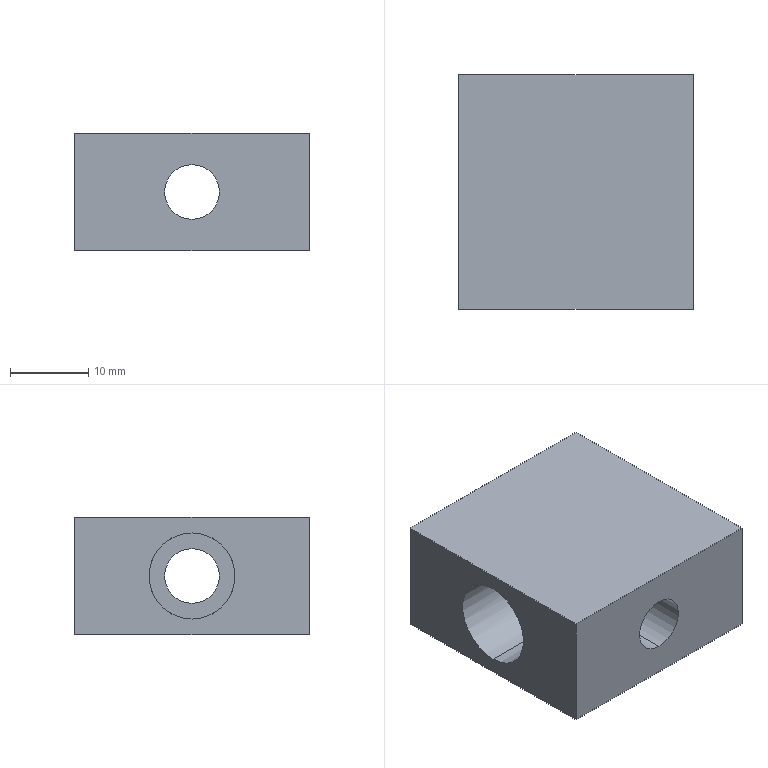Part | SolidWorks | features BaseBody 1 | 1 solid | 24 faces | box 30 x 30 x 15 mm | volume 9216 mm3 | cylinder 16 | plane 8 | commonest cylinder face diameters 11 x8 3.3 x4 7 x4
STEP:
#1=CARTESIAN_POINT('',(9.65,15.,2.));
#2=VERTEX_POINT('',#1);
#3=CARTESIAN_POINT('',(6.35,15.,2.));
#4=VERTEX_POINT('',#3);
#5=CARTESIAN_POINT('',(9.65,15.,2.));
#6=CARTESIAN_POINT('',(9.65,14.89,2.));
#7=CARTESIAN_POINT('',(9.639,14.783,2.003));
#8=CARTESIAN_POINT('',(9.597,14.571,2.016));
#9=CARTESIAN_POINT('',(9.565,14.466,2.025));
#10=CARTESIAN_POINT('',(9.482,14.266,2.048));
#11=CARTESIAN_POINT('',(9.431,14.172,2.062));
#12=CARTESIAN_POINT('',(9.311,13.993,2.092));
#13=CARTESIAN_POINT('',(9.242,13.909,2.109));
#14=CARTESIAN_POINT('',(9.015,13.682,2.158));
#15=CARTESIAN_POINT('',(8.832,13.559,2.191));
#16=CARTESIAN_POINT('',(8.436,13.394,2.239));
#17=CARTESIAN_POINT('',(8.218,13.35,2.253));
#18=CARTESIAN_POINT('',(7.893,13.35,2.253));
#19=CARTESIAN_POINT('',(7.783,13.361,2.25));
#20=CARTESIAN_POINT('',(7.571,13.403,2.237));
#21=CARTESIAN_POINT('',(7.468,13.434,2.227));
#22=CARTESIAN_POINT('',(7.167,13.559,2.191));
#23=CARTESIAN_POINT('',(6.986,13.681,2.158));
#24=CARTESIAN_POINT('',(6.758,13.909,2.109));
#25=CARTESIAN_POINT('',(6.69,13.991,2.093));
#26=CARTESIAN_POINT('',(6.57,14.169,2.062));
#27=CARTESIAN_POINT('',(6.518,14.266,2.048));
#28=CARTESIAN_POINT('',(6.394,14.564,2.014));
#29=CARTESIAN_POINT('',(6.35,14.781,2.));
#30=CARTESIAN_POINT('',(6.35,15.,2.));
#31=B_SPLINE_CURVE_WITH_KNOTS('',3,(#5,#6,#7,#8,#9,#10,#11,#12,#13,#14,#15,#16,#17,#18,#19,#20,#21,#22,#23,#24,#25,#26,#27,#28,#29,#30),.UNSPECIFIED.,.F.,.F.,(4,2,2,2,2,2,2,2,2,2,2,2,4),(0.,0.0003242,0.0006484,0.0009725,0.001297,0.001945,0.002593,0.002918,0.003242,0.00389,0.004214,0.004539,0.005187),.UNSPECIFIED.);
#32=EDGE_CURVE('',#2,#4,#31,.T.);
#33=ORIENTED_EDGE('',*,*,#32,.F.);
#34=CARTESIAN_POINT('',(9.65,15.,0.));
#35=VERTEX_POINT('',#34);
#36=CARTESIAN_POINT('',(9.65,15.,0.));
#37=DIRECTION('',(0.,0.,-1.));
#38=VECTOR('',#37,1000.);
#39=LINE('',#36,#38);
#40=EDGE_CURVE('',#2,#35,#39,.T.);
#41=ORIENTED_EDGE('',*,*,#40,.T.);
#42=CARTESIAN_POINT('',(6.35,15.,0.));
#43=VERTEX_POINT('',#42);
#44=CARTESIAN_POINT('',(8.,15.,0.));
#45=DIRECTION('',(0.,0.,-1.));
#46=DIRECTION('',(-1.,0.,0.));
#47=AXIS2_PLACEMENT_3D('',#44,#45,#46);
#48=CIRCLE('',#47,1.65);
#49=EDGE_CURVE('',#35,#43,#48,.T.);
#50=ORIENTED_EDGE('',*,*,#49,.T.);
#51=CARTESIAN_POINT('',(6.35,15.,0.));
#52=DIRECTION('',(0.,0.,-1.));
#53=VECTOR('',#52,1000.);
#54=LINE('',#51,#53);
#55=EDGE_CURVE('',#4,#43,#54,.T.);
#56=ORIENTED_EDGE('',*,*,#55,.F.);
#57=EDGE_LOOP('',(#33,#41,#50,#56));
#58=FACE_OUTER_BOUND('',#57,.T.);
#59=CARTESIAN_POINT('',(8.,15.,0.));
#60=DIRECTION('',(0.,0.,-1.));
#61=DIRECTION('',(-1.,0.,0.));
#62=AXIS2_PLACEMENT_3D('',#59,#60,#61);
#63=CYLINDRICAL_SURFACE('',#62,1.65);
#64=ADVANCED_FACE('',(#58),#63,.F.);
#65=CARTESIAN_POINT('',(16.65,22.,2.253));
#66=VERTEX_POINT('',#65);
#67=CARTESIAN_POINT('',(15.,20.35,2.));
#68=VERTEX_POINT('',#67);
#69=CARTESIAN_POINT('',(16.65,22.,2.253));
#70=CARTESIAN_POINT('',(16.65,21.89,2.253));
#71=CARTESIAN_POINT('',(16.639,21.783,2.25));
#72=CARTESIAN_POINT('',(16.597,21.571,2.237));
#73=CARTESIAN_POINT('',(16.565,21.466,2.227));
#74=CARTESIAN_POINT('',(16.482,21.267,2.203));
#75=CARTESIAN_POINT('',(16.431,21.172,2.189));
#76=CARTESIAN_POINT('',(16.312,20.993,2.158));
#77=CARTESIAN_POINT('',(16.243,20.909,2.142));
#78=CARTESIAN_POINT('',(16.016,20.682,2.092));
#79=CARTESIAN_POINT('',(15.833,20.56,2.06));
#80=CARTESIAN_POINT('',(15.437,20.394,2.014));
#81=CARTESIAN_POINT('',(15.219,20.35,2.));
#82=CARTESIAN_POINT('',(15.,20.35,2.));
#83=B_SPLINE_CURVE_WITH_KNOTS('',3,(#69,#70,#71,#72,#73,#74,#75,#76,#77,#78,#79,#80,#81,#82),.UNSPECIFIED.,.F.,.F.,(4,2,2,2,2,2,4),(0.,0.0003241,0.0006481,0.0009722,0.001296,0.001944,0.002593),.UNSPECIFIED.);
#84=EDGE_CURVE('',#66,#68,#83,.T.);
#85=ORIENTED_EDGE('',*,*,#84,.F.);
#86=CARTESIAN_POINT('',(16.65,22.,0.));
#87=VERTEX_POINT('',#86);
#88=CARTESIAN_POINT('',(16.65,22.,0.));
#89=DIRECTION('',(0.,0.,-1.));
#90=VECTOR('',#89,1000.);
#91=LINE('',#88,#90);
#92=EDGE_CURVE('',#66,#87,#91,.T.);
#93=ORIENTED_EDGE('',*,*,#92,.T.);
#94=CARTESIAN_POINT('',(13.35,22.,0.));
#95=VERTEX_POINT('',#94);
#96=CARTESIAN_POINT('',(15.,22.,0.));
#97=DIRECTION('',(0.,0.,-1.));
#98=DIRECTION('',(-1.,0.,0.));
#99=AXIS2_PLACEMENT_3D('',#96,#97,#98);
#100=CIRCLE('',#99,1.65);
#101=EDGE_CURVE('',#87,#95,#100,.T.);
#102=ORIENTED_EDGE('',*,*,#101,.T.);
#103=CARTESIAN_POINT('',(13.35,22.,2.253));
#104=VERTEX_POINT('',#103);
#105=CARTESIAN_POINT('',(13.35,22.,0.));
#106=DIRECTION('',(0.,0.,-1.));
#107=VECTOR('',#106,1000.);
#108=LINE('',#105,#107);
#109=EDGE_CURVE('',#104,#95,#108,.T.);
#110=ORIENTED_EDGE('',*,*,#109,.F.);
#111=CARTESIAN_POINT('',(15.,20.35,2.));
#112=CARTESIAN_POINT('',(14.89,20.35,2.));
#113=CARTESIAN_POINT('',(14.783,20.361,2.003));
#114=CARTESIAN_POINT('',(14.571,20.403,2.016));
#115=CARTESIAN_POINT('',(14.466,20.435,2.025));
#116=CARTESIAN_POINT('',(14.267,20.518,2.048));
#117=CARTESIAN_POINT('',(14.172,20.569,2.062));
#118=CARTESIAN_POINT('',(13.993,20.688,2.092));
#119=CARTESIAN_POINT('',(13.909,20.758,2.109));
#120=CARTESIAN_POINT('',(13.682,20.984,2.158));
#121=CARTESIAN_POINT('',(13.56,21.167,2.191));
#122=CARTESIAN_POINT('',(13.394,21.563,2.239));
#123=CARTESIAN_POINT('',(13.35,21.781,2.253));
#124=CARTESIAN_POINT('',(13.35,22.,2.253));
#125=B_SPLINE_CURVE_WITH_KNOTS('',3,(#111,#112,#113,#114,#115,#116,#117,#118,#119,#120,#121,#122,#123,#124),.UNSPECIFIED.,.F.,.F.,(4,2,2,2,2,2,4),(0.002593,0.002917,0.003241,0.003565,0.003889,0.004537,0.005185),.UNSPECIFIED.);
#126=EDGE_CURVE('',#68,#104,#125,.T.);
#127=ORIENTED_EDGE('',*,*,#126,.F.);
#128=EDGE_LOOP('',(#85,#93,#102,#110,#127));
#129=FACE_OUTER_BOUND('',#128,.T.);
#130=CARTESIAN_POINT('',(15.,22.,0.));
#131=DIRECTION('',(0.,0.,-1.));
#132=DIRECTION('',(-1.,0.,0.));
#133=AXIS2_PLACEMENT_3D('',#130,#131,#132);
#134=CYLINDRICAL_SURFACE('',#133,1.65);
#135=ADVANCED_FACE('',(#129),#134,.F.);
#136=CARTESIAN_POINT('',(30.,15.,4.));
#137=VERTEX_POINT('',#136);
#138=CARTESIAN_POINT('',(30.,15.,11.));
#139=VERTEX_POINT('',#138);
#140=CARTESIAN_POINT('',(30.,15.,7.5));
#141=DIRECTION('',(-1.,0.,0.));
#142=DIRECTION('',(0.,0.,1.));
#143=AXIS2_PLACEMENT_3D('',#140,#141,#142);
#144=CIRCLE('',#143,3.5);
#145=EDGE_CURVE('',#137,#139,#144,.T.);
#146=ORIENTED_EDGE('',*,*,#145,.F.);
#147=CARTESIAN_POINT('',(25.,15.,4.));
#148=VERTEX_POINT('',#147);
#149=CARTESIAN_POINT('',(0.,15.,4.));
#150=DIRECTION('',(-1.,0.,0.));
#151=VECTOR('',#150,1000.);
#152=LINE('',#149,#151);
#153=EDGE_CURVE('',#137,#148,#152,.T.);
#154=ORIENTED_EDGE('',*,*,#153,.T.);
#155=CARTESIAN_POINT('',(25.,15.,11.));
#156=VERTEX_POINT('',#155);
#157=CARTESIAN_POINT('',(25.,15.,7.5));
#158=DIRECTION('',(-1.,0.,0.));
#159=DIRECTION('',(0.,0.,1.));
#160=AXIS2_PLACEMENT_3D('',#157,#158,#159);
#161=CIRCLE('',#160,3.5);
#162=EDGE_CURVE('',#148,#156,#161,.T.);
#163=ORIENTED_EDGE('',*,*,#162,.T.);
#164=CARTESIAN_POINT('',(0.,15.,11.));
#165=DIRECTION('',(-1.,0.,0.));
#166=VECTOR('',#165,1000.);
#167=LINE('',#164,#166);
#168=EDGE_CURVE('',#139,#156,#167,.T.);
#169=ORIENTED_EDGE('',*,*,#168,.F.);
#170=EDGE_LOOP('',(#146,#154,#163,#169));
#171=FACE_OUTER_BOUND('',#170,.T.);
#172=CARTESIAN_POINT('',(0.,15.,7.5));
#173=DIRECTION('',(-1.,0.,0.));
#174=DIRECTION('',(0.,0.,1.));
#175=AXIS2_PLACEMENT_3D('',#172,#173,#174);
#176=CYLINDRICAL_SURFACE('',#175,3.5);
#177=ADVANCED_FACE('',(#171),#176,.F.);
#178=CARTESIAN_POINT('',(25.,15.,2.));
#179=VERTEX_POINT('',#178);
#180=CARTESIAN_POINT('',(25.,15.,13.));
#181=VERTEX_POINT('',#180);
#182=CARTESIAN_POINT('',(25.,15.,7.5));
#183=DIRECTION('',(-1.,0.,0.));
#184=DIRECTION('',(0.,0.,1.));
#185=AXIS2_PLACEMENT_3D('',#182,#183,#184);
#186=CIRCLE('',#185,5.5);
#187=EDGE_CURVE('',#179,#181,#186,.T.);
#188=ORIENTED_EDGE('',*,*,#187,.F.);
#189=CARTESIAN_POINT('',(15.,15.,2.));
#190=VERTEX_POINT('',#189);
#191=CARTESIAN_POINT('',(0.,15.,2.));
#192=DIRECTION('',(-1.,0.,0.));
#193=VECTOR('',#192,1000.);
#194=LINE('',#191,#193);
#195=EDGE_CURVE('',#179,#190,#194,.T.);
#196=ORIENTED_EDGE('',*,*,#195,.T.);
#197=CARTESIAN_POINT('',(15.,15.,13.));
#198=VERTEX_POINT('',#197);
#199=CARTESIAN_POINT('',(15.,15.,13.));
#200=CARTESIAN_POINT('',(26.,4.,13.));
#201=CARTESIAN_POINT('',(26.,4.,2.));
#202=CARTESIAN_POINT('',(15.,15.,2.));
#203=(BOUNDED_CURVE()B_SPLINE_CURVE(3,(#199,#200,#201,#202),.UNSPECIFIED.,.F.,.T.)B_SPLINE_CURVE_WITH_KNOTS((4,4),(1.571,4.712),.UNSPECIFIED.)CURVE()GEOMETRIC_REPRESENTATION_ITEM()RATIONAL_B_SPLINE_CURVE((1.,0.3333,0.3333,1.))REPRESENTATION_ITEM(''));
#204=EDGE_CURVE('',#198,#190,#203,.T.);
#205=ORIENTED_EDGE('',*,*,#204,.F.);
#206=CARTESIAN_POINT('',(0.,15.,13.));
#207=DIRECTION('',(-1.,0.,0.));
#208=VECTOR('',#207,1000.);
#209=LINE('',#206,#208);
#210=EDGE_CURVE('',#181,#198,#209,.T.);
#211=ORIENTED_EDGE('',*,*,#210,.F.);
#212=EDGE_LOOP('',(#188,#196,#205,#211));
#213=FACE_OUTER_BOUND('',#212,.T.);
#214=CARTESIAN_POINT('',(0.,15.,7.5));
#215=DIRECTION('',(-1.,0.,0.));
#216=DIRECTION('',(0.,0.,1.));
#217=AXIS2_PLACEMENT_3D('',#214,#215,#216);
#218=CYLINDRICAL_SURFACE('',#217,5.5);
#219=ADVANCED_FACE('',(#213),#218,.F.);
#220=CARTESIAN_POINT('',(15.,15.,2.));
#221=CARTESIAN_POINT('',(4.,4.,2.));
#222=CARTESIAN_POINT('',(4.,4.,13.));
#223=CARTESIAN_POINT('',(15.,15.,13.));
#224=(BOUNDED_CURVE()B_SPLINE_CURVE(3,(#220,#221,#222,#223),.UNSPECIFIED.,.F.,.F.)B_SPLINE_CURVE_WITH_KNOTS((4,4),(1.571,4.712),.UNSPECIFIED.)CURVE()GEOMETRIC_REPRESENTATION_ITEM()RATIONAL_B_SPLINE_CURVE((1.,0.3333,0.3333,1.))REPRESENTATION_ITEM(''));
#225=EDGE_CURVE('',#190,#198,#224,.T.);
#226=ORIENTED_EDGE('',*,*,#225,.F.);
#227=CARTESIAN_POINT('',(0.,15.,2.));
#228=DIRECTION('',(-1.,0.,0.));
#229=VECTOR('',#228,1000.);
#230=LINE('',#227,#229);
#231=EDGE_CURVE('',#190,#2,#230,.T.);
#232=ORIENTED_EDGE('',*,*,#231,.T.);
#233=ORIENTED_EDGE('',*,*,#32,.T.);
#234=CARTESIAN_POINT('',(0.,15.,2.));
#235=VERTEX_POINT('',#234);
#236=CARTESIAN_POINT('',(0.,15.,2.));
#237=DIRECTION('',(-1.,0.,0.));
#238=VECTOR('',#237,1000.);
#239=LINE('',#236,#238);
#240=EDGE_CURVE('',#4,#235,#239,.T.);
#241=ORIENTED_EDGE('',*,*,#240,.T.);
#242=CARTESIAN_POINT('',(0.,15.,13.));
#243=VERTEX_POINT('',#242);
#244=CARTESIAN_POINT('',(0.,15.,7.5));
#245=DIRECTION('',(-1.,0.,0.));
#246=DIRECTION('',(0.,0.,1.));
#247=AXIS2_PLACEMENT_3D('',#244,#245,#246);
#248=CIRCLE('',#247,5.5);
#249=EDGE_CURVE('',#235,#243,#248,.T.);
#250=ORIENTED_EDGE('',*,*,#249,.T.);
#251=CARTESIAN_POINT('',(0.,15.,13.));
#252=DIRECTION('',(-1.,0.,0.));
#253=VECTOR('',#252,1000.);
#254=LINE('',#251,#253);
#255=EDGE_CURVE('',#198,#243,#254,.T.);
#256=ORIENTED_EDGE('',*,*,#255,.F.);
#257=EDGE_LOOP('',(#226,#232,#233,#241,#250,#256));
#258=FACE_OUTER_BOUND('',#257,.T.);
#259=CARTESIAN_POINT('',(0.,15.,7.5));
#260=DIRECTION('',(-1.,0.,0.));
#261=DIRECTION('',(0.,0.,1.));
#262=AXIS2_PLACEMENT_3D('',#259,#260,#261);
#263=CYLINDRICAL_SURFACE('',#262,5.5);
#264=ADVANCED_FACE('',(#258),#263,.F.);
#265=CARTESIAN_POINT('',(15.,5.,2.));
#266=VERTEX_POINT('',#265);
#267=CARTESIAN_POINT('',(15.,5.,13.));
#268=VERTEX_POINT('',#267);
#269=CARTESIAN_POINT('',(15.,5.,7.5));
#270=DIRECTION('',(0.,1.,0.));
#271=DIRECTION('',(0.,0.,1.));
#272=AXIS2_PLACEMENT_3D('',#269,#270,#271);
#273=CIRCLE('',#272,5.5);
#274=EDGE_CURVE('',#266,#268,#273,.T.);
#275=ORIENTED_EDGE('',*,*,#274,.F.);
#276=CARTESIAN_POINT('',(15.,30.,2.));
#277=DIRECTION('',(0.,1.,0.));
#278=VECTOR('',#277,1000.);
#279=LINE('',#276,#278);
#280=EDGE_CURVE('',#266,#190,#279,.T.);
#281=ORIENTED_EDGE('',*,*,#280,.T.);
#282=ORIENTED_EDGE('',*,*,#225,.T.);
#283=CARTESIAN_POINT('',(15.,30.,13.));
#284=DIRECTION('',(0.,1.,0.));
#285=VECTOR('',#284,1000.);
#286=LINE('',#283,#285);
#287=EDGE_CURVE('',#268,#198,#286,.T.);
#288=ORIENTED_EDGE('',*,*,#287,.F.);
#289=EDGE_LOOP('',(#275,#281,#282,#288));
#290=FACE_OUTER_BOUND('',#289,.T.);
#291=CARTESIAN_POINT('',(15.,30.,7.5));
#292=DIRECTION('',(0.,1.,0.));
#293=DIRECTION('',(0.,0.,1.));
#294=AXIS2_PLACEMENT_3D('',#291,#292,#293);
#295=CYLINDRICAL_SURFACE('',#294,5.5);
#296=ADVANCED_FACE('',(#290),#295,.F.);
#297=CARTESIAN_POINT('',(15.,0.,4.));
#298=VERTEX_POINT('',#297);
#299=CARTESIAN_POINT('',(15.,0.,11.));
#300=VERTEX_POINT('',#299);
#301=CARTESIAN_POINT('',(15.,0.,7.5));
#302=DIRECTION('',(0.,1.,0.));
#303=DIRECTION('',(0.,0.,1.));
#304=AXIS2_PLACEMENT_3D('',#301,#302,#303);
#305=CIRCLE('',#304,3.5);
#306=EDGE_CURVE('',#298,#300,#305,.T.);
#307=ORIENTED_EDGE('',*,*,#306,.F.);
#308=CARTESIAN_POINT('',(15.,5.,4.));
#309=VERTEX_POINT('',#308);
#310=CARTESIAN_POINT('',(15.,30.,4.));
#311=DIRECTION('',(0.,1.,0.));
#312=VECTOR('',#311,1000.);
#313=LINE('',#310,#312);
#314=EDGE_CURVE('',#298,#309,#313,.T.);
#315=ORIENTED_EDGE('',*,*,#314,.T.);
#316=CARTESIAN_POINT('',(15.,5.,11.));
#317=VERTEX_POINT('',#316);
#318=CARTESIAN_POINT('',(15.,5.,7.5));
#319=DIRECTION('',(0.,1.,0.));
#320=DIRECTION('',(0.,0.,1.));
#321=AXIS2_PLACEMENT_3D('',#318,#319,#320);
#322=CIRCLE('',#321,3.5);
#323=EDGE_CURVE('',#309,#317,#322,.T.);
#324=ORIENTED_EDGE('',*,*,#323,.T.);
#325=CARTESIAN_POINT('',(15.,30.,11.));
#326=DIRECTION('',(0.,1.,0.));
#327=VECTOR('',#326,1000.);
#328=LINE('',#325,#327);
#329=EDGE_CURVE('',#300,#317,#328,.T.);
#330=ORIENTED_EDGE('',*,*,#329,.F.);
#331=EDGE_LOOP('',(#307,#315,#324,#330));
#332=FACE_OUTER_BOUND('',#331,.T.);
#333=CARTESIAN_POINT('',(15.,30.,7.5));
#334=DIRECTION('',(0.,1.,0.));
#335=DIRECTION('',(0.,0.,1.));
#336=AXIS2_PLACEMENT_3D('',#333,#334,#335);
#337=CYLINDRICAL_SURFACE('',#336,3.5);
#338=ADVANCED_FACE('',(#332),#337,.F.);
#339=CARTESIAN_POINT('',(15.,15.,13.));
#340=CARTESIAN_POINT('',(4.,26.,13.));
#341=CARTESIAN_POINT('',(4.,26.,2.));
#342=CARTESIAN_POINT('',(15.,15.,2.));
#343=(BOUNDED_CURVE()B_SPLINE_CURVE(3,(#339,#340,#341,#342),.UNSPECIFIED.,.F.,.F.)B_SPLINE_CURVE_WITH_KNOTS((4,4),(4.712,7.854),.UNSPECIFIED.)CURVE()GEOMETRIC_REPRESENTATION_ITEM()RATIONAL_B_SPLINE_CURVE((1.,0.3333,0.3333,1.))REPRESENTATION_ITEM(''));
#344=EDGE_CURVE('',#198,#190,#343,.T.);
#345=ORIENTED_EDGE('',*,*,#344,.T.);
#346=CARTESIAN_POINT('',(15.,30.,2.));
#347=DIRECTION('',(0.,1.,0.));
#348=VECTOR('',#347,1000.);
#349=LINE('',#346,#348);
#350=EDGE_CURVE('',#190,#68,#349,.T.);
#351=ORIENTED_EDGE('',*,*,#350,.T.);
#352=ORIENTED_EDGE('',*,*,#126,.T.);
#353=CARTESIAN_POINT('',(15.,23.65,2.));
#354=VERTEX_POINT('',#353);
#355=CARTESIAN_POINT('',(13.35,22.,2.253));
#356=CARTESIAN_POINT('',(13.35,22.11,2.253));
#357=CARTESIAN_POINT('',(13.361,22.217,2.25));
#358=CARTESIAN_POINT('',(13.403,22.429,2.237));
#359=CARTESIAN_POINT('',(13.435,22.534,2.227));
#360=CARTESIAN_POINT('',(13.518,22.733,2.203));
#361=CARTESIAN_POINT('',(13.569,22.828,2.189));
#362=CARTESIAN_POINT('',(13.688,23.007,2.158));
#363=CARTESIAN_POINT('',(13.757,23.091,2.142));
#364=CARTESIAN_POINT('',(13.984,23.318,2.092));
#365=CARTESIAN_POINT('',(14.167,23.44,2.06));
#366=CARTESIAN_POINT('',(14.563,23.606,2.014));
#367=CARTESIAN_POINT('',(14.781,23.65,2.));
#368=CARTESIAN_POINT('',(15.,23.65,2.));
#369=B_SPLINE_CURVE_WITH_KNOTS('',3,(#355,#356,#357,#358,#359,#360,#361,#362,#363,#364,#365,#366,#367,#368),.UNSPECIFIED.,.F.,.F.,(4,2,2,2,2,2,4),(0.005185,0.005509,0.005833,0.006157,0.006482,0.00713,0.007778),.UNSPECIFIED.);
#370=EDGE_CURVE('',#104,#354,#369,.T.);
#371=ORIENTED_EDGE('',*,*,#370,.T.);
#372=CARTESIAN_POINT('',(15.,30.,2.));
#373=VERTEX_POINT('',#372);
#374=CARTESIAN_POINT('',(15.,30.,2.));
#375=DIRECTION('',(0.,1.,0.));
#376=VECTOR('',#375,1000.);
#377=LINE('',#374,#376);
#378=EDGE_CURVE('',#354,#373,#377,.T.);
#379=ORIENTED_EDGE('',*,*,#378,.T.);
#380=CARTESIAN_POINT('',(15.,30.,13.));
#381=VERTEX_POINT('',#380);
#382=CARTESIAN_POINT('',(15.,30.,7.5));
#383=DIRECTION('',(0.,1.,0.));
#384=DIRECTION('',(0.,0.,1.));
#385=AXIS2_PLACEMENT_3D('',#382,#383,#384);
#386=CIRCLE('',#385,5.5);
#387=EDGE_CURVE('',#373,#381,#386,.T.);
#388=ORIENTED_EDGE('',*,*,#387,.T.);
#389=CARTESIAN_POINT('',(15.,30.,13.));
#390=DIRECTION('',(0.,1.,0.));
#391=VECTOR('',#390,1000.);
#392=LINE('',#389,#391);
#393=EDGE_CURVE('',#198,#381,#392,.T.);
#394=ORIENTED_EDGE('',*,*,#393,.F.);
#395=EDGE_LOOP('',(#345,#351,#352,#371,#379,#388,#394));
#396=FACE_OUTER_BOUND('',#395,.T.);
#397=CARTESIAN_POINT('',(15.,30.,7.5));
#398=DIRECTION('',(0.,1.,0.));
#399=DIRECTION('',(0.,0.,1.));
#400=AXIS2_PLACEMENT_3D('',#397,#398,#399);
#401=CYLINDRICAL_SURFACE('',#400,5.5);
#402=ADVANCED_FACE('',(#396),#401,.F.);
#403=CARTESIAN_POINT('',(25.,15.,7.5));
#404=DIRECTION('',(-1.,0.,0.));
#405=DIRECTION('',(0.,0.,1.));
#406=AXIS2_PLACEMENT_3D('',#403,#404,#405);
#407=CIRCLE('',#406,3.5);
#408=EDGE_CURVE('',#156,#148,#407,.T.);
#409=ORIENTED_EDGE('',*,*,#408,.F.);
#410=ORIENTED_EDGE('',*,*,#162,.F.);
#411=EDGE_LOOP('',(#409,#410));
#412=FACE_BOUND('',#411,.T.);
#413=CARTESIAN_POINT('',(25.,15.,7.5));
#414=DIRECTION('',(-1.,0.,0.));
#415=DIRECTION('',(0.,0.,1.));
#416=AXIS2_PLACEMENT_3D('',#413,#414,#415);
#417=CIRCLE('',#416,5.5);
#418=EDGE_CURVE('',#181,#179,#417,.T.);
#419=ORIENTED_EDGE('',*,*,#418,.T.);
#420=ORIENTED_EDGE('',*,*,#187,.T.);
#421=EDGE_LOOP('',(#419,#420));
#422=FACE_OUTER_BOUND('',#421,.T.);
#423=CARTESIAN_POINT('',(25.,18.5,7.5));
#424=DIRECTION('',(1.,0.,0.));
#425=DIRECTION('',(0.,1.,0.));
#426=AXIS2_PLACEMENT_3D('',#423,#424,#425);
#427=PLANE('',#426);
#428=ADVANCED_FACE('',(#412,#422),#427,.F.);
#429=CARTESIAN_POINT('',(15.,5.,7.5));
#430=DIRECTION('',(0.,1.,0.));
#431=DIRECTION('',(0.,0.,1.));
#432=AXIS2_PLACEMENT_3D('',#429,#430,#431);
#433=CIRCLE('',#432,3.5);
#434=EDGE_CURVE('',#317,#309,#433,.T.);
#435=ORIENTED_EDGE('',*,*,#434,.F.);
#436=ORIENTED_EDGE('',*,*,#323,.F.);
#437=EDGE_LOOP('',(#435,#436));
#438=FACE_BOUND('',#437,.T.);
#439=CARTESIAN_POINT('',(15.,5.,7.5));
#440=DIRECTION('',(0.,1.,0.));
#441=DIRECTION('',(0.,0.,1.));
#442=AXIS2_PLACEMENT_3D('',#439,#440,#441);
#443=CIRCLE('',#442,5.5);
#444=EDGE_CURVE('',#268,#266,#443,.T.);
#445=ORIENTED_EDGE('',*,*,#444,.T.);
#446=ORIENTED_EDGE('',*,*,#274,.T.);
#447=EDGE_LOOP('',(#445,#446));
#448=FACE_OUTER_BOUND('',#447,.T.);
#449=CARTESIAN_POINT('',(18.5,5.,7.5));
#450=DIRECTION('',(0.,-1.,0.));
#451=DIRECTION('',(0.,0.,-1.));
#452=AXIS2_PLACEMENT_3D('',#449,#450,#451);
#453=PLANE('',#452);
#454=ADVANCED_FACE('',(#438,#448),#453,.F.);
#455=CARTESIAN_POINT('',(15.,22.,0.));
#456=DIRECTION('',(0.,0.,-1.));
#457=DIRECTION('',(-1.,0.,0.));
#458=AXIS2_PLACEMENT_3D('',#455,#456,#457);
#459=CIRCLE('',#458,1.65);
#460=EDGE_CURVE('',#95,#87,#459,.T.);
#461=ORIENTED_EDGE('',*,*,#460,.F.);
#462=ORIENTED_EDGE('',*,*,#101,.F.);
#463=EDGE_LOOP('',(#461,#462));
#464=FACE_BOUND('',#463,.T.);
#465=CARTESIAN_POINT('',(8.,15.,0.));
#466=DIRECTION('',(0.,0.,-1.));
#467=DIRECTION('',(-1.,0.,0.));
#468=AXIS2_PLACEMENT_3D('',#465,#466,#467);
#469=CIRCLE('',#468,1.65);
#470=EDGE_CURVE('',#43,#35,#469,.T.);
#471=ORIENTED_EDGE('',*,*,#470,.F.);
#472=ORIENTED_EDGE('',*,*,#49,.F.);
#473=EDGE_LOOP('',(#471,#472));
#474=FACE_BOUND('',#473,.T.);
#475=CARTESIAN_POINT('',(0.,30.,0.));
#476=VERTEX_POINT('',#475);
#477=CARTESIAN_POINT('',(0.,0.,0.));
#478=VERTEX_POINT('',#477);
#479=CARTESIAN_POINT('',(0.,0.,0.));
#480=DIRECTION('',(0.,-1.,0.));
#481=VECTOR('',#480,1000.);
#482=LINE('',#479,#481);
#483=EDGE_CURVE('',#476,#478,#482,.T.);
#484=ORIENTED_EDGE('',*,*,#483,.F.);
#485=CARTESIAN_POINT('',(30.,30.,0.));
#486=VERTEX_POINT('',#485);
#487=CARTESIAN_POINT('',(0.,30.,0.));
#488=DIRECTION('',(-1.,0.,0.));
#489=VECTOR('',#488,1000.);
#490=LINE('',#487,#489);
#491=EDGE_CURVE('',#486,#476,#490,.T.);
#492=ORIENTED_EDGE('',*,*,#491,.F.);
#493=CARTESIAN_POINT('',(30.,0.,0.));
#494=VERTEX_POINT('',#493);
#495=CARTESIAN_POINT('',(30.,0.,0.));
#496=DIRECTION('',(0.,1.,0.));
#497=VECTOR('',#496,1000.);
#498=LINE('',#495,#497);
#499=EDGE_CURVE('',#494,#486,#498,.T.);
#500=ORIENTED_EDGE('',*,*,#499,.F.);
#501=CARTESIAN_POINT('',(0.,0.,0.));
#502=DIRECTION('',(1.,0.,0.));
#503=VECTOR('',#502,1000.);
#504=LINE('',#501,#503);
#505=EDGE_CURVE('',#478,#494,#504,.T.);
#506=ORIENTED_EDGE('',*,*,#505,.F.);
#507=EDGE_LOOP('',(#484,#492,#500,#506));
#508=FACE_OUTER_BOUND('',#507,.T.);
#509=CARTESIAN_POINT('',(0.,0.,0.));
#510=DIRECTION('',(0.,0.,-1.));
#511=DIRECTION('',(0.,-1.,0.));
#512=AXIS2_PLACEMENT_3D('',#509,#510,#511);
#513=PLANE('',#512);
#514=ADVANCED_FACE('',(#464,#474,#508),#513,.T.);
#515=CARTESIAN_POINT('',(0.,30.,15.));
#516=VERTEX_POINT('',#515);
#517=CARTESIAN_POINT('',(0.,0.,15.));
#518=VERTEX_POINT('',#517);
#519=CARTESIAN_POINT('',(0.,0.,15.));
#520=DIRECTION('',(0.,-1.,0.));
#521=VECTOR('',#520,1000.);
#522=LINE('',#519,#521);
#523=EDGE_CURVE('',#516,#518,#522,.T.);
#524=ORIENTED_EDGE('',*,*,#523,.T.);
#525=CARTESIAN_POINT('',(30.,0.,15.));
#526=VERTEX_POINT('',#525);
#527=CARTESIAN_POINT('',(0.,0.,15.));
#528=DIRECTION('',(1.,0.,0.));
#529=VECTOR('',#528,1000.);
#530=LINE('',#527,#529);
#531=EDGE_CURVE('',#518,#526,#530,.T.);
#532=ORIENTED_EDGE('',*,*,#531,.T.);
#533=CARTESIAN_POINT('',(30.,30.,15.));
#534=VERTEX_POINT('',#533);
#535=CARTESIAN_POINT('',(30.,0.,15.));
#536=DIRECTION('',(0.,1.,0.));
#537=VECTOR('',#536,1000.);
#538=LINE('',#535,#537);
#539=EDGE_CURVE('',#526,#534,#538,.T.);
#540=ORIENTED_EDGE('',*,*,#539,.T.);
#541=CARTESIAN_POINT('',(0.,30.,15.));
#542=DIRECTION('',(-1.,0.,0.));
#543=VECTOR('',#542,1000.);
#544=LINE('',#541,#543);
#545=EDGE_CURVE('',#534,#516,#544,.T.);
#546=ORIENTED_EDGE('',*,*,#545,.T.);
#547=EDGE_LOOP('',(#524,#532,#540,#546));
#548=FACE_OUTER_BOUND('',#547,.T.);
#549=CARTESIAN_POINT('',(0.,0.,15.));
#550=DIRECTION('',(0.,0.,-1.));
#551=DIRECTION('',(0.,-1.,0.));
#552=AXIS2_PLACEMENT_3D('',#549,#550,#551);
#553=PLANE('',#552);
#554=ADVANCED_FACE('',(#548),#553,.F.);
#555=CARTESIAN_POINT('',(15.,30.,7.5));
#556=DIRECTION('',(0.,1.,0.));
#557=DIRECTION('',(0.,0.,1.));
#558=AXIS2_PLACEMENT_3D('',#555,#556,#557);
#559=CIRCLE('',#558,5.5);
#560=EDGE_CURVE('',#381,#373,#559,.T.);
#561=ORIENTED_EDGE('',*,*,#560,.F.);
#562=ORIENTED_EDGE('',*,*,#387,.F.);
#563=EDGE_LOOP('',(#561,#562));
#564=FACE_BOUND('',#563,.T.);
#565=ORIENTED_EDGE('',*,*,#491,.T.);
#566=CARTESIAN_POINT('',(0.,30.,15.));
#567=DIRECTION('',(0.,0.,-1.));
#568=VECTOR('',#567,1000.);
#569=LINE('',#566,#568);
#570=EDGE_CURVE('',#516,#476,#569,.T.);
#571=ORIENTED_EDGE('',*,*,#570,.F.);
#572=ORIENTED_EDGE('',*,*,#545,.F.);
#573=CARTESIAN_POINT('',(30.,30.,15.));
#574=DIRECTION('',(0.,0.,-1.));
#575=VECTOR('',#574,1000.);
#576=LINE('',#573,#575);
#577=EDGE_CURVE('',#534,#486,#576,.T.);
#578=ORIENTED_EDGE('',*,*,#577,.T.);
#579=EDGE_LOOP('',(#565,#571,#572,#578));
#580=FACE_OUTER_BOUND('',#579,.T.);
#581=CARTESIAN_POINT('',(0.,30.,15.));
#582=DIRECTION('',(0.,-1.,0.));
#583=DIRECTION('',(0.,0.,-1.));
#584=AXIS2_PLACEMENT_3D('',#581,#582,#583);
#585=PLANE('',#584);
#586=ADVANCED_FACE('',(#564,#580),#585,.F.);
#587=CARTESIAN_POINT('',(30.,15.,7.5));
#588=DIRECTION('',(-1.,0.,0.));
#589=DIRECTION('',(0.,0.,1.));
#590=AXIS2_PLACEMENT_3D('',#587,#588,#589);
#591=CIRCLE('',#590,3.5);
#592=EDGE_CURVE('',#139,#137,#591,.T.);
#593=ORIENTED_EDGE('',*,*,#592,.T.);
#594=ORIENTED_EDGE('',*,*,#145,.T.);
#595=EDGE_LOOP('',(#593,#594));
#596=FACE_BOUND('',#595,.T.);
#597=ORIENTED_EDGE('',*,*,#499,.T.);
#598=ORIENTED_EDGE('',*,*,#577,.F.);
#599=ORIENTED_EDGE('',*,*,#539,.F.);
#600=CARTESIAN_POINT('',(30.,0.,15.));
#601=DIRECTION('',(0.,0.,-1.));
#602=VECTOR('',#601,1000.);
#603=LINE('',#600,#602);
#604=EDGE_CURVE('',#526,#494,#603,.T.);
#605=ORIENTED_EDGE('',*,*,#604,.T.);
#606=EDGE_LOOP('',(#597,#598,#599,#605));
#607=FACE_OUTER_BOUND('',#606,.T.);
#608=CARTESIAN_POINT('',(30.,0.,15.));
#609=DIRECTION('',(-1.,0.,0.));
#610=DIRECTION('',(0.,0.,1.));
#611=AXIS2_PLACEMENT_3D('',#608,#609,#610);
#612=PLANE('',#611);
#613=ADVANCED_FACE('',(#596,#607),#612,.F.);
#614=CARTESIAN_POINT('',(15.,0.,7.5));
#615=DIRECTION('',(0.,1.,0.));
#616=DIRECTION('',(0.,0.,1.));
#617=AXIS2_PLACEMENT_3D('',#614,#615,#616);
#618=CIRCLE('',#617,3.5);
#619=EDGE_CURVE('',#300,#298,#618,.T.);
#620=ORIENTED_EDGE('',*,*,#619,.T.);
#621=ORIENTED_EDGE('',*,*,#306,.T.);
#622=EDGE_LOOP('',(#620,#621));
#623=FACE_BOUND('',#622,.T.);
#624=ORIENTED_EDGE('',*,*,#505,.T.);
#625=ORIENTED_EDGE('',*,*,#604,.F.);
#626=ORIENTED_EDGE('',*,*,#531,.F.);
#627=CARTESIAN_POINT('',(0.,0.,15.));
#628=DIRECTION('',(0.,0.,-1.));
#629=VECTOR('',#628,1000.);
#630=LINE('',#627,#629);
#631=EDGE_CURVE('',#518,#478,#630,.T.);
#632=ORIENTED_EDGE('',*,*,#631,.T.);
#633=EDGE_LOOP('',(#624,#625,#626,#632));
#634=FACE_OUTER_BOUND('',#633,.T.);
#635=CARTESIAN_POINT('',(0.,0.,15.));
#636=DIRECTION('',(0.,1.,0.));
#637=DIRECTION('',(1.,0.,0.));
#638=AXIS2_PLACEMENT_3D('',#635,#636,#637);
#639=PLANE('',#638);
#640=ADVANCED_FACE('',(#623,#634),#639,.F.);
#641=CARTESIAN_POINT('',(0.,15.,7.5));
#642=DIRECTION('',(-1.,0.,0.));
#643=DIRECTION('',(0.,0.,1.));
#644=AXIS2_PLACEMENT_3D('',#641,#642,#643);
#645=CIRCLE('',#644,5.5);
#646=EDGE_CURVE('',#243,#235,#645,.T.);
#647=ORIENTED_EDGE('',*,*,#646,.F.);
#648=ORIENTED_EDGE('',*,*,#249,.F.);
#649=EDGE_LOOP('',(#647,#648));
#650=FACE_BOUND('',#649,.T.);
#651=ORIENTED_EDGE('',*,*,#483,.T.);
#652=ORIENTED_EDGE('',*,*,#631,.F.);
#653=ORIENTED_EDGE('',*,*,#523,.F.);
#654=ORIENTED_EDGE('',*,*,#570,.T.);
#655=EDGE_LOOP('',(#651,#652,#653,#654));
#656=FACE_OUTER_BOUND('',#655,.T.);
#657=CARTESIAN_POINT('',(0.,0.,15.));
#658=DIRECTION('',(1.,0.,0.));
#659=DIRECTION('',(0.,1.,0.));
#660=AXIS2_PLACEMENT_3D('',#657,#658,#659);
#661=PLANE('',#660);
#662=ADVANCED_FACE('',(#650,#656),#661,.F.);
#663=ORIENTED_EDGE('',*,*,#350,.F.);
#664=CARTESIAN_POINT('',(15.,15.,2.));
#665=CARTESIAN_POINT('',(26.,26.,2.));
#666=CARTESIAN_POINT('',(26.,26.,13.));
#667=CARTESIAN_POINT('',(15.,15.,13.));
#668=(BOUNDED_CURVE()B_SPLINE_CURVE(3,(#664,#665,#666,#667),.UNSPECIFIED.,.F.,.F.)B_SPLINE_CURVE_WITH_KNOTS((4,4),(4.712,7.854),.UNSPECIFIED.)CURVE()GEOMETRIC_REPRESENTATION_ITEM()RATIONAL_B_SPLINE_CURVE((1.,0.3333,0.3333,1.))REPRESENTATION_ITEM(''));
#669=EDGE_CURVE('',#190,#198,#668,.T.);
#670=ORIENTED_EDGE('',*,*,#669,.T.);
#671=ORIENTED_EDGE('',*,*,#393,.T.);
#672=ORIENTED_EDGE('',*,*,#560,.T.);
#673=ORIENTED_EDGE('',*,*,#378,.F.);
#674=CARTESIAN_POINT('',(15.,23.65,2.));
#675=CARTESIAN_POINT('',(15.11,23.65,2.));
#676=CARTESIAN_POINT('',(15.217,23.639,2.003));
#677=CARTESIAN_POINT('',(15.429,23.597,2.016));
#678=CARTESIAN_POINT('',(15.534,23.565,2.025));
#679=CARTESIAN_POINT('',(15.733,23.482,2.048));
#680=CARTESIAN_POINT('',(15.828,23.431,2.062));
#681=CARTESIAN_POINT('',(16.007,23.312,2.092));
#682=CARTESIAN_POINT('',(16.091,23.242,2.109));
#683=CARTESIAN_POINT('',(16.318,23.016,2.158));
#684=CARTESIAN_POINT('',(16.44,22.833,2.191));
#685=CARTESIAN_POINT('',(16.606,22.437,2.239));
#686=CARTESIAN_POINT('',(16.65,22.219,2.253));
#687=CARTESIAN_POINT('',(16.65,22.,2.253));
#688=B_SPLINE_CURVE_WITH_KNOTS('',3,(#674,#675,#676,#677,#678,#679,#680,#681,#682,#683,#684,#685,#686,#687),.UNSPECIFIED.,.F.,.F.,(4,2,2,2,2,2,4),(0.007778,0.008102,0.008426,0.00875,0.009074,0.009722,0.01037),.UNSPECIFIED.);
#689=EDGE_CURVE('',#354,#66,#688,.T.);
#690=ORIENTED_EDGE('',*,*,#689,.T.);
#691=ORIENTED_EDGE('',*,*,#84,.T.);
#692=EDGE_LOOP('',(#663,#670,#671,#672,#673,#690,#691));
#693=FACE_OUTER_BOUND('',#692,.T.);
#694=CARTESIAN_POINT('',(15.,30.,7.5));
#695=DIRECTION('',(0.,1.,0.));
#696=DIRECTION('',(0.,0.,1.));
#697=AXIS2_PLACEMENT_3D('',#694,#695,#696);
#698=CYLINDRICAL_SURFACE('',#697,5.5);
#699=ADVANCED_FACE('',(#693),#698,.F.);
#700=ORIENTED_EDGE('',*,*,#314,.F.);
#701=ORIENTED_EDGE('',*,*,#619,.F.);
#702=ORIENTED_EDGE('',*,*,#329,.T.);
#703=ORIENTED_EDGE('',*,*,#434,.T.);
#704=EDGE_LOOP('',(#700,#701,#702,#703));
#705=FACE_OUTER_BOUND('',#704,.T.);
#706=CARTESIAN_POINT('',(15.,30.,7.5));
#707=DIRECTION('',(0.,1.,0.));
#708=DIRECTION('',(0.,0.,1.));
#709=AXIS2_PLACEMENT_3D('',#706,#707,#708);
#710=CYLINDRICAL_SURFACE('',#709,3.5);
#711=ADVANCED_FACE('',(#705),#710,.F.);
#712=ORIENTED_EDGE('',*,*,#280,.F.);
#713=ORIENTED_EDGE('',*,*,#444,.F.);
#714=ORIENTED_EDGE('',*,*,#287,.T.);
#715=ORIENTED_EDGE('',*,*,#204,.T.);
#716=EDGE_LOOP('',(#712,#713,#714,#715));
#717=FACE_OUTER_BOUND('',#716,.T.);
#718=CARTESIAN_POINT('',(15.,30.,7.5));
#719=DIRECTION('',(0.,1.,0.));
#720=DIRECTION('',(0.,0.,1.));
#721=AXIS2_PLACEMENT_3D('',#718,#719,#720);
#722=CYLINDRICAL_SURFACE('',#721,5.5);
#723=ADVANCED_FACE('',(#717),#722,.F.);
#724=ORIENTED_EDGE('',*,*,#231,.F.);
#725=ORIENTED_EDGE('',*,*,#344,.F.);
#726=ORIENTED_EDGE('',*,*,#255,.T.);
#727=ORIENTED_EDGE('',*,*,#646,.T.);
#728=ORIENTED_EDGE('',*,*,#240,.F.);
#729=CARTESIAN_POINT('',(6.35,15.,2.));
#730=CARTESIAN_POINT('',(6.35,15.11,2.));
#731=CARTESIAN_POINT('',(6.361,15.217,2.003));
#732=CARTESIAN_POINT('',(6.403,15.429,2.016));
#733=CARTESIAN_POINT('',(6.435,15.534,2.025));
#734=CARTESIAN_POINT('',(6.518,15.734,2.048));
#735=CARTESIAN_POINT('',(6.569,15.828,2.062));
#736=CARTESIAN_POINT('',(6.689,16.007,2.092));
#737=CARTESIAN_POINT('',(6.758,16.091,2.109));
#738=CARTESIAN_POINT('',(6.985,16.318,2.158));
#739=CARTESIAN_POINT('',(7.168,16.441,2.191));
#740=CARTESIAN_POINT('',(7.564,16.606,2.239));
#741=CARTESIAN_POINT('',(7.782,16.65,2.253));
#742=CARTESIAN_POINT('',(8.107,16.65,2.253));
#743=CARTESIAN_POINT('',(8.217,16.639,2.25));
#744=CARTESIAN_POINT('',(8.429,16.597,2.237));
#745=CARTESIAN_POINT('',(8.532,16.566,2.227));
#746=CARTESIAN_POINT('',(8.833,16.441,2.191));
#747=CARTESIAN_POINT('',(9.014,16.319,2.158));
#748=CARTESIAN_POINT('',(9.242,16.091,2.109));
#749=CARTESIAN_POINT('',(9.31,16.009,2.093));
#750=CARTESIAN_POINT('',(9.43,15.831,2.062));
#751=CARTESIAN_POINT('',(9.482,15.734,2.048));
#752=CARTESIAN_POINT('',(9.606,15.436,2.014));
#753=CARTESIAN_POINT('',(9.65,15.219,2.));
#754=CARTESIAN_POINT('',(9.65,15.,2.));
#755=B_SPLINE_CURVE_WITH_KNOTS('',3,(#729,#730,#731,#732,#733,#734,#735,#736,#737,#738,#739,#740,#741,#742,#743,#744,#745,#746,#747,#748,#749,#750,#751,#752,#753,#754),.UNSPECIFIED.,.F.,.F.,(4,2,2,2,2,2,2,2,2,2,2,2,4),(0.005187,0.005511,0.005835,0.006159,0.006484,0.007132,0.00778,0.008104,0.008428,0.009077,0.009401,0.009725,0.01037),.UNSPECIFIED.);
#756=EDGE_CURVE('',#4,#2,#755,.T.);
#757=ORIENTED_EDGE('',*,*,#756,.T.);
#758=EDGE_LOOP('',(#724,#725,#726,#727,#728,#757));
#759=FACE_OUTER_BOUND('',#758,.T.);
#760=CARTESIAN_POINT('',(0.,15.,7.5));
#761=DIRECTION('',(-1.,0.,0.));
#762=DIRECTION('',(0.,0.,1.));
#763=AXIS2_PLACEMENT_3D('',#760,#761,#762);
#764=CYLINDRICAL_SURFACE('',#763,5.5);
#765=ADVANCED_FACE('',(#759),#764,.F.);
#766=ORIENTED_EDGE('',*,*,#195,.F.);
#767=ORIENTED_EDGE('',*,*,#418,.F.);
#768=ORIENTED_EDGE('',*,*,#210,.T.);
#769=ORIENTED_EDGE('',*,*,#669,.F.);
#770=EDGE_LOOP('',(#766,#767,#768,#769));
#771=FACE_OUTER_BOUND('',#770,.T.);
#772=CARTESIAN_POINT('',(0.,15.,7.5));
#773=DIRECTION('',(-1.,0.,0.));
#774=DIRECTION('',(0.,0.,1.));
#775=AXIS2_PLACEMENT_3D('',#772,#773,#774);
#776=CYLINDRICAL_SURFACE('',#775,5.5);
#777=ADVANCED_FACE('',(#771),#776,.F.);
#778=ORIENTED_EDGE('',*,*,#153,.F.);
#779=ORIENTED_EDGE('',*,*,#592,.F.);
#780=ORIENTED_EDGE('',*,*,#168,.T.);
#781=ORIENTED_EDGE('',*,*,#408,.T.);
#782=EDGE_LOOP('',(#778,#779,#780,#781));
#783=FACE_OUTER_BOUND('',#782,.T.);
#784=CARTESIAN_POINT('',(0.,15.,7.5));
#785=DIRECTION('',(-1.,0.,0.));
#786=DIRECTION('',(0.,0.,1.));
#787=AXIS2_PLACEMENT_3D('',#784,#785,#786);
#788=CYLINDRICAL_SURFACE('',#787,3.5);
#789=ADVANCED_FACE('',(#783),#788,.F.);
#790=ORIENTED_EDGE('',*,*,#92,.F.);
#791=ORIENTED_EDGE('',*,*,#689,.F.);
#792=ORIENTED_EDGE('',*,*,#370,.F.);
#793=ORIENTED_EDGE('',*,*,#109,.T.);
#794=ORIENTED_EDGE('',*,*,#460,.T.);
#795=EDGE_LOOP('',(#790,#791,#792,#793,#794));
#796=FACE_OUTER_BOUND('',#795,.T.);
#797=CARTESIAN_POINT('',(15.,22.,0.));
#798=DIRECTION('',(0.,0.,-1.));
#799=DIRECTION('',(-1.,0.,0.));
#800=AXIS2_PLACEMENT_3D('',#797,#798,#799);
#801=CYLINDRICAL_SURFACE('',#800,1.65);
#802=ADVANCED_FACE('',(#796),#801,.F.);
#803=ORIENTED_EDGE('',*,*,#40,.F.);
#804=ORIENTED_EDGE('',*,*,#756,.F.);
#805=ORIENTED_EDGE('',*,*,#55,.T.);
#806=ORIENTED_EDGE('',*,*,#470,.T.);
#807=EDGE_LOOP('',(#803,#804,#805,#806));
#808=FACE_OUTER_BOUND('',#807,.T.);
#809=CARTESIAN_POINT('',(8.,15.,0.));
#810=DIRECTION('',(0.,0.,-1.));
#811=DIRECTION('',(-1.,0.,0.));
#812=AXIS2_PLACEMENT_3D('',#809,#810,#811);
#813=CYLINDRICAL_SURFACE('',#812,1.65);
#814=ADVANCED_FACE('',(#808),#813,.F.);
#815=CLOSED_SHELL('',(#64,#135,#177,#219,#264,#296,#338,#402,#428,#454,#514,#554,#586,#613,#640,#662,#699,#711,#723,#765,#777,#789,#802,#814));
#816=MANIFOLD_SOLID_BREP('',#815);
#817=CARTESIAN_POINT('',(0.,0.,0.));
#818=DIRECTION('',(0.,0.,1.));
#819=DIRECTION('',(1.,0.,0.));
#820=AXIS2_PLACEMENT_3D('',#817,#818,#819);
#821=(LENGTH_UNIT()NAMED_UNIT(*)SI_UNIT(.MILLI.,.METRE.));
#822=UNCERTAINTY_MEASURE_WITH_UNIT(LENGTH_MEASURE(0.00001),#821,'','');
#823=(NAMED_UNIT(*)PLANE_ANGLE_UNIT()SI_UNIT($,.RADIAN.));
#824=(NAMED_UNIT(*)SI_UNIT($,.STERADIAN.)SOLID_ANGLE_UNIT());
#825=(GEOMETRIC_REPRESENTATION_CONTEXT(3)GLOBAL_UNCERTAINTY_ASSIGNED_CONTEXT((#822))GLOBAL_UNIT_ASSIGNED_CONTEXT((#821,#823,#824))REPRESENTATION_CONTEXT('',''));
#826=ADVANCED_BREP_SHAPE_REPRESENTATION('',(#816,#820),#825);